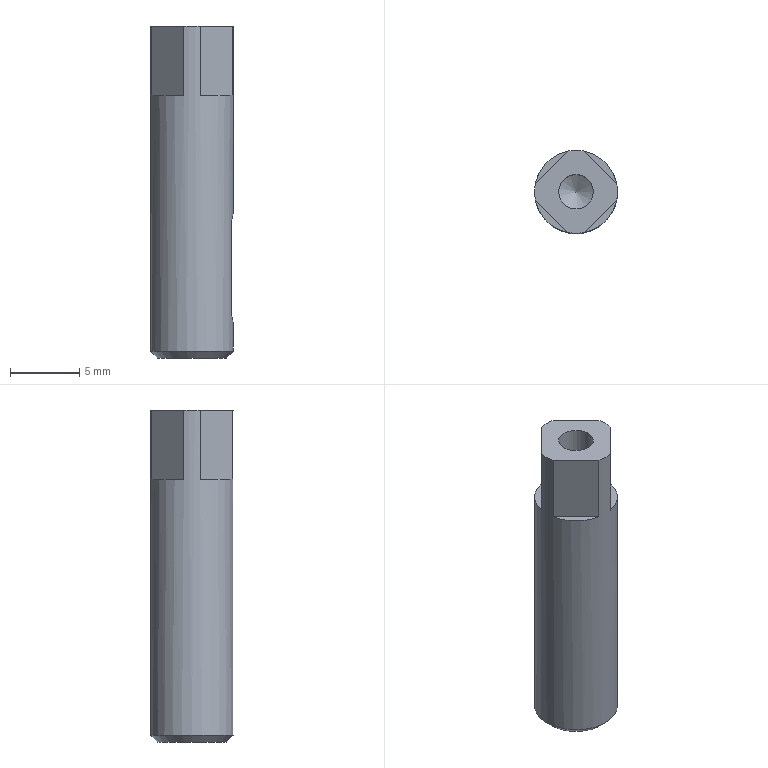Part | NX | features BREP 1 | 1 solid | 20 faces | box 6 x 6 x 24 mm | volume 581.313 mm3 | plane 13 | cylinder 5 | cone 2 | commonest cylinder face diameters 2 x2 2.5 x2 6 x1
STEP:
#1=CARTESIAN_POINT('',(-0.5952,-2.94,19.));
#2=VERTEX_POINT('',#1);
#3=CARTESIAN_POINT('',(-2.94,-0.5952,19.));
#4=VERTEX_POINT('',#3);
#5=CARTESIAN_POINT('',(-0.5952,-2.94,19.));
#6=DIRECTION('',(-0.7071,0.7071,0.));
#7=VECTOR('',#6,1000.);
#8=LINE('',#5,#7);
#9=EDGE_CURVE('',#2,#4,#8,.T.);
#10=ORIENTED_EDGE('',*,*,#9,.T.);
#11=CARTESIAN_POINT('',(0.,0.,19.));
#12=DIRECTION('',(0.,0.,1.));
#13=DIRECTION('',(-0.9801,-0.1984,0.));
#14=AXIS2_PLACEMENT_3D('',#11,#12,#13);
#15=CIRCLE('',#14,3.);
#16=EDGE_CURVE('',#4,#2,#15,.T.);
#17=ORIENTED_EDGE('',*,*,#16,.T.);
#18=EDGE_LOOP('',(#10,#17));
#19=FACE_BOUND('',#18,.T.);
#20=CARTESIAN_POINT('',(0.,0.,19.));
#21=DIRECTION('',(0.,0.,1.));
#22=DIRECTION('',(-1.,0.,0.));
#23=AXIS2_PLACEMENT_3D('',#20,#21,#22);
#24=PLANE('',#23);
#25=ADVANCED_FACE('',(#19),#24,.T.);
#26=CARTESIAN_POINT('',(2.94,-0.5952,19.));
#27=VERTEX_POINT('',#26);
#28=CARTESIAN_POINT('',(0.5952,-2.94,19.));
#29=VERTEX_POINT('',#28);
#30=CARTESIAN_POINT('',(2.94,-0.5952,19.));
#31=DIRECTION('',(-0.7071,-0.7071,0.));
#32=VECTOR('',#31,1000.);
#33=LINE('',#30,#32);
#34=EDGE_CURVE('',#27,#29,#33,.T.);
#35=ORIENTED_EDGE('',*,*,#34,.T.);
#36=CARTESIAN_POINT('',(0.,0.,19.));
#37=DIRECTION('',(0.,0.,1.));
#38=DIRECTION('',(0.1984,-0.9801,0.));
#39=AXIS2_PLACEMENT_3D('',#36,#37,#38);
#40=CIRCLE('',#39,3.);
#41=EDGE_CURVE('',#29,#27,#40,.T.);
#42=ORIENTED_EDGE('',*,*,#41,.T.);
#43=EDGE_LOOP('',(#35,#42));
#44=FACE_BOUND('',#43,.T.);
#45=CARTESIAN_POINT('',(0.,0.,19.));
#46=DIRECTION('',(0.,0.,1.));
#47=DIRECTION('',(-1.,0.,0.));
#48=AXIS2_PLACEMENT_3D('',#45,#46,#47);
#49=PLANE('',#48);
#50=ADVANCED_FACE('',(#44),#49,.T.);
#51=CARTESIAN_POINT('',(0.5952,2.94,19.));
#52=VERTEX_POINT('',#51);
#53=CARTESIAN_POINT('',(2.94,0.5952,19.));
#54=VERTEX_POINT('',#53);
#55=CARTESIAN_POINT('',(0.5952,2.94,19.));
#56=DIRECTION('',(0.7071,-0.7071,0.));
#57=VECTOR('',#56,1000.);
#58=LINE('',#55,#57);
#59=EDGE_CURVE('',#52,#54,#58,.T.);
#60=ORIENTED_EDGE('',*,*,#59,.T.);
#61=CARTESIAN_POINT('',(0.,0.,19.));
#62=DIRECTION('',(0.,0.,1.));
#63=DIRECTION('',(0.9801,0.1984,0.));
#64=AXIS2_PLACEMENT_3D('',#61,#62,#63);
#65=CIRCLE('',#64,3.);
#66=EDGE_CURVE('',#54,#52,#65,.T.);
#67=ORIENTED_EDGE('',*,*,#66,.T.);
#68=EDGE_LOOP('',(#60,#67));
#69=FACE_BOUND('',#68,.T.);
#70=CARTESIAN_POINT('',(0.,0.,19.));
#71=DIRECTION('',(0.,0.,1.));
#72=DIRECTION('',(-1.,0.,0.));
#73=AXIS2_PLACEMENT_3D('',#70,#71,#72);
#74=PLANE('',#73);
#75=ADVANCED_FACE('',(#69),#74,.T.);
#76=CARTESIAN_POINT('',(-2.94,0.5952,19.));
#77=VERTEX_POINT('',#76);
#78=CARTESIAN_POINT('',(-0.5952,2.94,19.));
#79=VERTEX_POINT('',#78);
#80=CARTESIAN_POINT('',(-2.94,0.5952,19.));
#81=DIRECTION('',(0.7071,0.7071,0.));
#82=VECTOR('',#81,1000.);
#83=LINE('',#80,#82);
#84=EDGE_CURVE('',#77,#79,#83,.T.);
#85=ORIENTED_EDGE('',*,*,#84,.T.);
#86=CARTESIAN_POINT('',(0.,0.,19.));
#87=DIRECTION('',(0.,0.,1.));
#88=DIRECTION('',(-0.1984,0.9801,0.));
#89=AXIS2_PLACEMENT_3D('',#86,#87,#88);
#90=CIRCLE('',#89,3.);
#91=EDGE_CURVE('',#79,#77,#90,.T.);
#92=ORIENTED_EDGE('',*,*,#91,.T.);
#93=EDGE_LOOP('',(#85,#92));
#94=FACE_BOUND('',#93,.T.);
#95=CARTESIAN_POINT('',(0.,0.,19.));
#96=DIRECTION('',(0.,0.,1.));
#97=DIRECTION('',(-1.,0.,0.));
#98=AXIS2_PLACEMENT_3D('',#95,#96,#97);
#99=PLANE('',#98);
#100=ADVANCED_FACE('',(#94),#99,.T.);
#101=CARTESIAN_POINT('',(-0.5952,-2.94,24.));
#102=VERTEX_POINT('',#101);
#103=CARTESIAN_POINT('',(-2.94,-0.5952,24.));
#104=VERTEX_POINT('',#103);
#105=CARTESIAN_POINT('',(-0.5952,-2.94,24.));
#106=DIRECTION('',(-0.7071,0.7071,0.));
#107=VECTOR('',#106,1000.);
#108=LINE('',#105,#107);
#109=EDGE_CURVE('',#102,#104,#108,.T.);
#110=ORIENTED_EDGE('',*,*,#109,.T.);
#111=CARTESIAN_POINT('',(-2.94,-0.5952,24.));
#112=DIRECTION('',(0.,0.,-1.));
#113=VECTOR('',#112,1000.);
#114=LINE('',#111,#113);
#115=EDGE_CURVE('',#104,#4,#114,.T.);
#116=ORIENTED_EDGE('',*,*,#115,.T.);
#117=ORIENTED_EDGE('',*,*,#9,.F.);
#118=CARTESIAN_POINT('',(-0.5952,-2.94,19.));
#119=DIRECTION('',(0.,0.,1.));
#120=VECTOR('',#119,1000.);
#121=LINE('',#118,#120);
#122=EDGE_CURVE('',#2,#102,#121,.T.);
#123=ORIENTED_EDGE('',*,*,#122,.T.);
#124=EDGE_LOOP('',(#110,#116,#117,#123));
#125=FACE_BOUND('',#124,.T.);
#126=CARTESIAN_POINT('',(-1.768,-1.768,21.5));
#127=DIRECTION('',(-0.7071,-0.7071,0.));
#128=DIRECTION('',(0.7071,-0.7071,0.));
#129=AXIS2_PLACEMENT_3D('',#126,#127,#128);
#130=PLANE('',#129);
#131=ADVANCED_FACE('',(#125),#130,.T.);
#132=CARTESIAN_POINT('',(-2.94,0.5952,24.));
#133=VERTEX_POINT('',#132);
#134=CARTESIAN_POINT('',(-0.5952,2.94,24.));
#135=VERTEX_POINT('',#134);
#136=CARTESIAN_POINT('',(-2.94,0.5952,24.));
#137=DIRECTION('',(0.7071,0.7071,0.));
#138=VECTOR('',#137,1000.);
#139=LINE('',#136,#138);
#140=EDGE_CURVE('',#133,#135,#139,.T.);
#141=ORIENTED_EDGE('',*,*,#140,.T.);
#142=CARTESIAN_POINT('',(-0.5952,2.94,24.));
#143=DIRECTION('',(0.,0.,-1.));
#144=VECTOR('',#143,1000.);
#145=LINE('',#142,#144);
#146=EDGE_CURVE('',#135,#79,#145,.T.);
#147=ORIENTED_EDGE('',*,*,#146,.T.);
#148=ORIENTED_EDGE('',*,*,#84,.F.);
#149=CARTESIAN_POINT('',(-2.94,0.5952,19.));
#150=DIRECTION('',(0.,0.,1.));
#151=VECTOR('',#150,1000.);
#152=LINE('',#149,#151);
#153=EDGE_CURVE('',#77,#133,#152,.T.);
#154=ORIENTED_EDGE('',*,*,#153,.T.);
#155=EDGE_LOOP('',(#141,#147,#148,#154));
#156=FACE_BOUND('',#155,.T.);
#157=CARTESIAN_POINT('',(-1.768,1.768,21.5));
#158=DIRECTION('',(-0.7071,0.7071,0.));
#159=DIRECTION('',(-0.7071,-0.7071,0.));
#160=AXIS2_PLACEMENT_3D('',#157,#158,#159);
#161=PLANE('',#160);
#162=ADVANCED_FACE('',(#156),#161,.T.);
#163=CARTESIAN_POINT('',(0.5952,2.94,24.));
#164=VERTEX_POINT('',#163);
#165=CARTESIAN_POINT('',(2.94,0.5952,24.));
#166=VERTEX_POINT('',#165);
#167=CARTESIAN_POINT('',(0.5952,2.94,24.));
#168=DIRECTION('',(0.7071,-0.7071,0.));
#169=VECTOR('',#168,1000.);
#170=LINE('',#167,#169);
#171=EDGE_CURVE('',#164,#166,#170,.T.);
#172=ORIENTED_EDGE('',*,*,#171,.T.);
#173=CARTESIAN_POINT('',(2.94,0.5952,24.));
#174=DIRECTION('',(0.,0.,-1.));
#175=VECTOR('',#174,1000.);
#176=LINE('',#173,#175);
#177=EDGE_CURVE('',#166,#54,#176,.T.);
#178=ORIENTED_EDGE('',*,*,#177,.T.);
#179=ORIENTED_EDGE('',*,*,#59,.F.);
#180=CARTESIAN_POINT('',(0.5952,2.94,19.));
#181=DIRECTION('',(0.,0.,1.));
#182=VECTOR('',#181,1000.);
#183=LINE('',#180,#182);
#184=EDGE_CURVE('',#52,#164,#183,.T.);
#185=ORIENTED_EDGE('',*,*,#184,.T.);
#186=EDGE_LOOP('',(#172,#178,#179,#185));
#187=FACE_BOUND('',#186,.T.);
#188=CARTESIAN_POINT('',(1.768,1.768,21.5));
#189=DIRECTION('',(0.7071,0.7071,0.));
#190=DIRECTION('',(-0.7071,0.7071,0.));
#191=AXIS2_PLACEMENT_3D('',#188,#189,#190);
#192=PLANE('',#191);
#193=ADVANCED_FACE('',(#187),#192,.T.);
#194=CARTESIAN_POINT('',(2.94,-0.5952,24.));
#195=VERTEX_POINT('',#194);
#196=CARTESIAN_POINT('',(0.5952,-2.94,24.));
#197=VERTEX_POINT('',#196);
#198=CARTESIAN_POINT('',(2.94,-0.5952,24.));
#199=DIRECTION('',(-0.7071,-0.7071,0.));
#200=VECTOR('',#199,1000.);
#201=LINE('',#198,#200);
#202=EDGE_CURVE('',#195,#197,#201,.T.);
#203=ORIENTED_EDGE('',*,*,#202,.T.);
#204=CARTESIAN_POINT('',(0.5952,-2.94,24.));
#205=DIRECTION('',(0.,0.,-1.));
#206=VECTOR('',#205,1000.);
#207=LINE('',#204,#206);
#208=EDGE_CURVE('',#197,#29,#207,.T.);
#209=ORIENTED_EDGE('',*,*,#208,.T.);
#210=ORIENTED_EDGE('',*,*,#34,.F.);
#211=CARTESIAN_POINT('',(2.94,-0.5952,19.));
#212=DIRECTION('',(0.,0.,1.));
#213=VECTOR('',#212,1000.);
#214=LINE('',#211,#213);
#215=EDGE_CURVE('',#27,#195,#214,.T.);
#216=ORIENTED_EDGE('',*,*,#215,.T.);
#217=EDGE_LOOP('',(#203,#209,#210,#216));
#218=FACE_BOUND('',#217,.T.);
#219=CARTESIAN_POINT('',(1.768,-1.768,21.5));
#220=DIRECTION('',(0.7071,-0.7071,0.));
#221=DIRECTION('',(0.7071,0.7071,0.));
#222=AXIS2_PLACEMENT_3D('',#219,#220,#221);
#223=PLANE('',#222);
#224=ADVANCED_FACE('',(#218),#223,.T.);
#225=CARTESIAN_POINT('',(3.,0.,24.));
#226=VERTEX_POINT('',#225);
#227=CARTESIAN_POINT('',(0.,0.,24.));
#228=DIRECTION('',(0.,0.,1.));
#229=DIRECTION('',(0.9801,-0.1984,0.));
#230=AXIS2_PLACEMENT_3D('',#227,#228,#229);
#231=CIRCLE('',#230,3.);
#232=EDGE_CURVE('',#195,#226,#231,.T.);
#233=ORIENTED_EDGE('',*,*,#232,.F.);
#234=ORIENTED_EDGE('',*,*,#215,.F.);
#235=ORIENTED_EDGE('',*,*,#41,.F.);
#236=ORIENTED_EDGE('',*,*,#208,.F.);
#237=CARTESIAN_POINT('',(0.,0.,24.));
#238=DIRECTION('',(0.,0.,1.));
#239=DIRECTION('',(-0.1984,-0.9801,0.));
#240=AXIS2_PLACEMENT_3D('',#237,#238,#239);
#241=CIRCLE('',#240,3.);
#242=EDGE_CURVE('',#102,#197,#241,.T.);
#243=ORIENTED_EDGE('',*,*,#242,.F.);
#244=ORIENTED_EDGE('',*,*,#122,.F.);
#245=ORIENTED_EDGE('',*,*,#16,.F.);
#246=ORIENTED_EDGE('',*,*,#115,.F.);
#247=CARTESIAN_POINT('',(0.,0.,24.));
#248=DIRECTION('',(0.,0.,1.));
#249=DIRECTION('',(-0.9801,0.1984,0.));
#250=AXIS2_PLACEMENT_3D('',#247,#248,#249);
#251=CIRCLE('',#250,3.);
#252=EDGE_CURVE('',#133,#104,#251,.T.);
#253=ORIENTED_EDGE('',*,*,#252,.F.);
#254=ORIENTED_EDGE('',*,*,#153,.F.);
#255=ORIENTED_EDGE('',*,*,#91,.F.);
#256=ORIENTED_EDGE('',*,*,#146,.F.);
#257=CARTESIAN_POINT('',(0.,0.,24.));
#258=DIRECTION('',(0.,0.,1.));
#259=DIRECTION('',(0.1984,0.9801,0.));
#260=AXIS2_PLACEMENT_3D('',#257,#258,#259);
#261=CIRCLE('',#260,3.);
#262=EDGE_CURVE('',#164,#135,#261,.T.);
#263=ORIENTED_EDGE('',*,*,#262,.F.);
#264=ORIENTED_EDGE('',*,*,#184,.F.);
#265=ORIENTED_EDGE('',*,*,#66,.F.);
#266=ORIENTED_EDGE('',*,*,#177,.F.);
#267=CARTESIAN_POINT('',(0.,0.,24.));
#268=DIRECTION('',(0.,0.,1.));
#269=DIRECTION('',(1.,0.,0.));
#270=AXIS2_PLACEMENT_3D('',#267,#268,#269);
#271=CIRCLE('',#270,3.);
#272=EDGE_CURVE('',#226,#166,#271,.T.);
#273=ORIENTED_EDGE('',*,*,#272,.F.);
#274=CARTESIAN_POINT('',(3.,0.,10.5));
#275=VERTEX_POINT('',#274);
#276=CARTESIAN_POINT('',(3.,0.,10.5));
#277=DIRECTION('',(0.,0.,1.));
#278=VECTOR('',#277,1000.);
#279=LINE('',#276,#278);
#280=EDGE_CURVE('',#275,#226,#279,.T.);
#281=ORIENTED_EDGE('',*,*,#280,.F.);
#282=CARTESIAN_POINT('',(2.828,1.,9.5));
#283=VERTEX_POINT('',#282);
#284=CARTESIAN_POINT('',(2.828,1.,9.5));
#285=CARTESIAN_POINT('',(2.828,1.,10.032));
#286=CARTESIAN_POINT('',(3.,0.5323,10.5));
#287=CARTESIAN_POINT('',(3.,0.,10.5));
#288=B_SPLINE_CURVE_WITH_KNOTS('',3,(#284,#285,#286,#287),.UNSPECIFIED.,.F.,.F.,(4,4),(0.,0.001574),.UNSPECIFIED.);
#289=EDGE_CURVE('',#283,#275,#288,.T.);
#290=ORIENTED_EDGE('',*,*,#289,.F.);
#291=CARTESIAN_POINT('',(2.828,1.,3.5));
#292=VERTEX_POINT('',#291);
#293=CARTESIAN_POINT('',(2.828,1.,3.5));
#294=DIRECTION('',(0.,0.,1.));
#295=VECTOR('',#294,1000.);
#296=LINE('',#293,#295);
#297=EDGE_CURVE('',#292,#283,#296,.T.);
#298=ORIENTED_EDGE('',*,*,#297,.F.);
#299=CARTESIAN_POINT('',(3.,0.,2.5));
#300=VERTEX_POINT('',#299);
#301=CARTESIAN_POINT('',(3.,0.,2.5));
#302=CARTESIAN_POINT('',(3.,0.5323,2.5));
#303=CARTESIAN_POINT('',(2.828,1.,2.968));
#304=CARTESIAN_POINT('',(2.828,1.,3.5));
#305=B_SPLINE_CURVE_WITH_KNOTS('',3,(#301,#302,#303,#304),.UNSPECIFIED.,.F.,.F.,(4,4),(0.,0.001574),.UNSPECIFIED.);
#306=EDGE_CURVE('',#300,#292,#305,.T.);
#307=ORIENTED_EDGE('',*,*,#306,.F.);
#308=CARTESIAN_POINT('',(3.,0.,0.5));
#309=VERTEX_POINT('',#308);
#310=CARTESIAN_POINT('',(3.,0.,0.5));
#311=DIRECTION('',(0.,0.,1.));
#312=VECTOR('',#311,1000.);
#313=LINE('',#310,#312);
#314=EDGE_CURVE('',#309,#300,#313,.T.);
#315=ORIENTED_EDGE('',*,*,#314,.F.);
#316=CARTESIAN_POINT('',(0.,0.,0.5));
#317=DIRECTION('',(0.,0.,-1.));
#318=DIRECTION('',(1.,0.,0.));
#319=AXIS2_PLACEMENT_3D('',#316,#317,#318);
#320=CIRCLE('',#319,3.);
#321=EDGE_CURVE('',#309,#309,#320,.T.);
#322=ORIENTED_EDGE('',*,*,#321,.F.);
#323=ORIENTED_EDGE('',*,*,#314,.T.);
#324=CARTESIAN_POINT('',(2.828,-1.,3.5));
#325=VERTEX_POINT('',#324);
#326=CARTESIAN_POINT('',(2.828,-1.,3.5));
#327=CARTESIAN_POINT('',(2.828,-1.,2.968));
#328=CARTESIAN_POINT('',(3.,-0.5323,2.5));
#329=CARTESIAN_POINT('',(3.,0.,2.5));
#330=B_SPLINE_CURVE_WITH_KNOTS('',3,(#326,#327,#328,#329),.UNSPECIFIED.,.F.,.F.,(4,4),(0.,0.001574),.UNSPECIFIED.);
#331=EDGE_CURVE('',#325,#300,#330,.T.);
#332=ORIENTED_EDGE('',*,*,#331,.F.);
#333=CARTESIAN_POINT('',(2.828,-1.,9.5));
#334=VERTEX_POINT('',#333);
#335=CARTESIAN_POINT('',(2.828,-1.,9.5));
#336=DIRECTION('',(0.,0.,-1.));
#337=VECTOR('',#336,1000.);
#338=LINE('',#335,#337);
#339=EDGE_CURVE('',#334,#325,#338,.T.);
#340=ORIENTED_EDGE('',*,*,#339,.F.);
#341=CARTESIAN_POINT('',(3.,0.,10.5));
#342=CARTESIAN_POINT('',(3.,-0.5323,10.5));
#343=CARTESIAN_POINT('',(2.828,-1.,10.032));
#344=CARTESIAN_POINT('',(2.828,-1.,9.5));
#345=B_SPLINE_CURVE_WITH_KNOTS('',3,(#341,#342,#343,#344),.UNSPECIFIED.,.F.,.F.,(4,4),(0.,0.001574),.UNSPECIFIED.);
#346=EDGE_CURVE('',#275,#334,#345,.T.);
#347=ORIENTED_EDGE('',*,*,#346,.F.);
#348=ORIENTED_EDGE('',*,*,#280,.T.);
#349=EDGE_LOOP('',(#233,#234,#235,#236,#243,#244,#245,#246,#253,#254,#255,#256,#263,#264,#265,#266,#273,#281,#290,#298,#307,#315,#322,#323,#332,#340,#347,#348));
#350=FACE_BOUND('',#349,.T.);
#351=CARTESIAN_POINT('',(0.,0.,0.));
#352=DIRECTION('',(0.,0.,1.));
#353=DIRECTION('',(-1.,0.,0.));
#354=AXIS2_PLACEMENT_3D('',#351,#352,#353);
#355=CYLINDRICAL_SURFACE('',#354,3.);
#356=ADVANCED_FACE('',(#350),#355,.T.);
#357=ORIENTED_EDGE('',*,*,#272,.T.);
#358=ORIENTED_EDGE('',*,*,#171,.F.);
#359=ORIENTED_EDGE('',*,*,#262,.T.);
#360=ORIENTED_EDGE('',*,*,#140,.F.);
#361=ORIENTED_EDGE('',*,*,#252,.T.);
#362=ORIENTED_EDGE('',*,*,#109,.F.);
#363=ORIENTED_EDGE('',*,*,#242,.T.);
#364=ORIENTED_EDGE('',*,*,#202,.F.);
#365=ORIENTED_EDGE('',*,*,#232,.T.);
#366=EDGE_LOOP('',(#357,#358,#359,#360,#361,#362,#363,#364,#365));
#367=FACE_BOUND('',#366,.T.);
#368=CARTESIAN_POINT('',(1.25,0.,24.));
#369=VERTEX_POINT('',#368);
#370=CARTESIAN_POINT('',(0.,0.,24.));
#371=DIRECTION('',(0.,0.,-1.));
#372=DIRECTION('',(1.,0.,0.));
#373=AXIS2_PLACEMENT_3D('',#370,#371,#372);
#374=CIRCLE('',#373,1.25);
#375=EDGE_CURVE('',#369,#369,#374,.T.);
#376=ORIENTED_EDGE('',*,*,#375,.T.);
#377=EDGE_LOOP('',(#376));
#378=FACE_BOUND('',#377,.T.);
#379=CARTESIAN_POINT('',(0.,0.,24.));
#380=DIRECTION('',(0.,0.,1.));
#381=DIRECTION('',(-1.,0.,0.));
#382=AXIS2_PLACEMENT_3D('',#379,#380,#381);
#383=PLANE('',#382);
#384=ADVANCED_FACE('',(#367,#378),#383,.T.);
#385=CARTESIAN_POINT('',(2.5,0.,0.));
#386=VERTEX_POINT('',#385);
#387=CARTESIAN_POINT('',(0.,0.,0.));
#388=DIRECTION('',(0.,0.,-1.));
#389=DIRECTION('',(1.,0.,0.));
#390=AXIS2_PLACEMENT_3D('',#387,#388,#389);
#391=CIRCLE('',#390,2.5);
#392=EDGE_CURVE('',#386,#386,#391,.T.);
#393=ORIENTED_EDGE('',*,*,#392,.T.);
#394=EDGE_LOOP('',(#393));
#395=FACE_BOUND('',#394,.T.);
#396=CARTESIAN_POINT('',(0.,0.,0.));
#397=DIRECTION('',(0.,0.,1.));
#398=DIRECTION('',(-1.,0.,0.));
#399=AXIS2_PLACEMENT_3D('',#396,#397,#398);
#400=PLANE('',#399);
#401=ADVANCED_FACE('',(#395),#400,.F.);
#402=ORIENTED_EDGE('',*,*,#392,.F.);
#403=CARTESIAN_POINT('',(2.5,0.,0.));
#404=DIRECTION('',(0.7071,0.,0.7071));
#405=VECTOR('',#404,1000.);
#406=LINE('',#403,#405);
#407=EDGE_CURVE('',#386,#309,#406,.T.);
#408=ORIENTED_EDGE('',*,*,#407,.T.);
#409=ORIENTED_EDGE('',*,*,#321,.T.);
#410=ORIENTED_EDGE('',*,*,#407,.F.);
#411=EDGE_LOOP('',(#402,#408,#409,#410));
#412=FACE_BOUND('',#411,.T.);
#413=CARTESIAN_POINT('',(0.,0.,0.));
#414=DIRECTION('',(0.,0.,1.));
#415=DIRECTION('',(-1.,0.,0.));
#416=AXIS2_PLACEMENT_3D('',#413,#414,#415);
#417=CONICAL_SURFACE('',#416,2.5,0.7854);
#418=ADVANCED_FACE('',(#412),#417,.T.);
#419=CARTESIAN_POINT('',(1.8,1.,9.5));
#420=VERTEX_POINT('',#419);
#421=CARTESIAN_POINT('',(1.8,1.,9.5));
#422=DIRECTION('',(1.,0.,0.));
#423=VECTOR('',#422,1000.);
#424=LINE('',#421,#423);
#425=EDGE_CURVE('',#420,#283,#424,.T.);
#426=ORIENTED_EDGE('',*,*,#425,.T.);
#427=ORIENTED_EDGE('',*,*,#289,.T.);
#428=ORIENTED_EDGE('',*,*,#346,.T.);
#429=CARTESIAN_POINT('',(1.8,-1.,9.5));
#430=VERTEX_POINT('',#429);
#431=CARTESIAN_POINT('',(1.8,-1.,9.5));
#432=DIRECTION('',(1.,0.,0.));
#433=VECTOR('',#432,1000.);
#434=LINE('',#431,#433);
#435=EDGE_CURVE('',#430,#334,#434,.T.);
#436=ORIENTED_EDGE('',*,*,#435,.F.);
#437=CARTESIAN_POINT('',(1.8,0.,9.5));
#438=DIRECTION('',(1.,0.,0.));
#439=DIRECTION('',(0.,1.,0.));
#440=AXIS2_PLACEMENT_3D('',#437,#438,#439);
#441=CIRCLE('',#440,1.);
#442=EDGE_CURVE('',#420,#430,#441,.T.);
#443=ORIENTED_EDGE('',*,*,#442,.F.);
#444=EDGE_LOOP('',(#426,#427,#428,#436,#443));
#445=FACE_BOUND('',#444,.T.);
#446=CARTESIAN_POINT('',(1.8,0.,9.5));
#447=DIRECTION('',(1.,0.,0.));
#448=DIRECTION('',(0.,-1.,0.));
#449=AXIS2_PLACEMENT_3D('',#446,#447,#448);
#450=CYLINDRICAL_SURFACE('',#449,1.);
#451=ADVANCED_FACE('',(#445),#450,.F.);
#452=CARTESIAN_POINT('',(1.8,1.,3.5));
#453=VERTEX_POINT('',#452);
#454=CARTESIAN_POINT('',(1.8,1.,3.5));
#455=DIRECTION('',(1.,0.,0.));
#456=VECTOR('',#455,1000.);
#457=LINE('',#454,#456);
#458=EDGE_CURVE('',#453,#292,#457,.T.);
#459=ORIENTED_EDGE('',*,*,#458,.T.);
#460=ORIENTED_EDGE('',*,*,#297,.T.);
#461=ORIENTED_EDGE('',*,*,#425,.F.);
#462=CARTESIAN_POINT('',(1.8,1.,3.5));
#463=DIRECTION('',(0.,0.,1.));
#464=VECTOR('',#463,1000.);
#465=LINE('',#462,#464);
#466=EDGE_CURVE('',#453,#420,#465,.T.);
#467=ORIENTED_EDGE('',*,*,#466,.F.);
#468=EDGE_LOOP('',(#459,#460,#461,#467));
#469=FACE_BOUND('',#468,.T.);
#470=CARTESIAN_POINT('',(4.805,1.,6.5));
#471=DIRECTION('',(0.,1.,0.));
#472=DIRECTION('',(0.,0.,-1.));
#473=AXIS2_PLACEMENT_3D('',#470,#471,#472);
#474=PLANE('',#473);
#475=ADVANCED_FACE('',(#469),#474,.F.);
#476=CARTESIAN_POINT('',(1.8,-1.,3.5));
#477=VERTEX_POINT('',#476);
#478=CARTESIAN_POINT('',(1.8,-1.,3.5));
#479=DIRECTION('',(1.,0.,0.));
#480=VECTOR('',#479,1000.);
#481=LINE('',#478,#480);
#482=EDGE_CURVE('',#477,#325,#481,.T.);
#483=ORIENTED_EDGE('',*,*,#482,.T.);
#484=ORIENTED_EDGE('',*,*,#331,.T.);
#485=ORIENTED_EDGE('',*,*,#306,.T.);
#486=ORIENTED_EDGE('',*,*,#458,.F.);
#487=CARTESIAN_POINT('',(1.8,0.,3.5));
#488=DIRECTION('',(1.,0.,0.));
#489=DIRECTION('',(0.,-1.,0.));
#490=AXIS2_PLACEMENT_3D('',#487,#488,#489);
#491=CIRCLE('',#490,1.);
#492=EDGE_CURVE('',#477,#453,#491,.T.);
#493=ORIENTED_EDGE('',*,*,#492,.F.);
#494=EDGE_LOOP('',(#483,#484,#485,#486,#493));
#495=FACE_BOUND('',#494,.T.);
#496=CARTESIAN_POINT('',(1.8,0.,3.5));
#497=DIRECTION('',(1.,0.,0.));
#498=DIRECTION('',(0.,1.,0.));
#499=AXIS2_PLACEMENT_3D('',#496,#497,#498);
#500=CYLINDRICAL_SURFACE('',#499,1.);
#501=ADVANCED_FACE('',(#495),#500,.F.);
#502=ORIENTED_EDGE('',*,*,#435,.T.);
#503=ORIENTED_EDGE('',*,*,#339,.T.);
#504=ORIENTED_EDGE('',*,*,#482,.F.);
#505=CARTESIAN_POINT('',(1.8,-1.,9.5));
#506=DIRECTION('',(0.,0.,-1.));
#507=VECTOR('',#506,1000.);
#508=LINE('',#505,#507);
#509=EDGE_CURVE('',#430,#477,#508,.T.);
#510=ORIENTED_EDGE('',*,*,#509,.F.);
#511=EDGE_LOOP('',(#502,#503,#504,#510));
#512=FACE_BOUND('',#511,.T.);
#513=CARTESIAN_POINT('',(4.805,-1.,6.5));
#514=DIRECTION('',(0.,-1.,0.));
#515=DIRECTION('',(0.,0.,1.));
#516=AXIS2_PLACEMENT_3D('',#513,#514,#515);
#517=PLANE('',#516);
#518=ADVANCED_FACE('',(#512),#517,.F.);
#519=ORIENTED_EDGE('',*,*,#442,.T.);
#520=ORIENTED_EDGE('',*,*,#509,.T.);
#521=ORIENTED_EDGE('',*,*,#492,.T.);
#522=ORIENTED_EDGE('',*,*,#466,.T.);
#523=EDGE_LOOP('',(#519,#520,#521,#522));
#524=FACE_BOUND('',#523,.T.);
#525=CARTESIAN_POINT('',(1.8,3.,6.5));
#526=DIRECTION('',(1.,0.,0.));
#527=DIRECTION('',(0.,-1.,0.));
#528=AXIS2_PLACEMENT_3D('',#525,#526,#527);
#529=PLANE('',#528);
#530=ADVANCED_FACE('',(#524),#529,.T.);
#531=CARTESIAN_POINT('',(1.25,0.,15.));
#532=VERTEX_POINT('',#531);
#533=CARTESIAN_POINT('',(1.25,0.,24.));
#534=DIRECTION('',(0.,0.,-1.));
#535=VECTOR('',#534,1000.);
#536=LINE('',#533,#535);
#537=EDGE_CURVE('',#369,#532,#536,.T.);
#538=ORIENTED_EDGE('',*,*,#537,.T.);
#539=CARTESIAN_POINT('',(0.,0.,15.));
#540=DIRECTION('',(0.,0.,-1.));
#541=DIRECTION('',(1.,0.,0.));
#542=AXIS2_PLACEMENT_3D('',#539,#540,#541);
#543=CIRCLE('',#542,1.25);
#544=EDGE_CURVE('',#532,#532,#543,.T.);
#545=ORIENTED_EDGE('',*,*,#544,.T.);
#546=ORIENTED_EDGE('',*,*,#537,.F.);
#547=ORIENTED_EDGE('',*,*,#375,.F.);
#548=EDGE_LOOP('',(#538,#545,#546,#547));
#549=FACE_BOUND('',#548,.T.);
#550=CARTESIAN_POINT('',(0.,0.,24.));
#551=DIRECTION('',(0.,0.,-1.));
#552=DIRECTION('',(-1.,0.,0.));
#553=AXIS2_PLACEMENT_3D('',#550,#551,#552);
#554=CYLINDRICAL_SURFACE('',#553,1.25);
#555=ADVANCED_FACE('',(#549),#554,.F.);
#556=CARTESIAN_POINT('',(1.25,0.,13.));
#557=VERTEX_POINT('',#556);
#558=CARTESIAN_POINT('',(1.25,0.,15.));
#559=DIRECTION('',(0.,0.,-1.));
#560=VECTOR('',#559,1000.);
#561=LINE('',#558,#560);
#562=EDGE_CURVE('',#532,#557,#561,.T.);
#563=ORIENTED_EDGE('',*,*,#562,.T.);
#564=CARTESIAN_POINT('',(0.,0.,13.));
#565=DIRECTION('',(0.,0.,-1.));
#566=DIRECTION('',(1.,0.,0.));
#567=AXIS2_PLACEMENT_3D('',#564,#565,#566);
#568=CIRCLE('',#567,1.25);
#569=EDGE_CURVE('',#557,#557,#568,.T.);
#570=ORIENTED_EDGE('',*,*,#569,.T.);
#571=ORIENTED_EDGE('',*,*,#562,.F.);
#572=ORIENTED_EDGE('',*,*,#544,.F.);
#573=EDGE_LOOP('',(#563,#570,#571,#572));
#574=FACE_BOUND('',#573,.T.);
#575=CARTESIAN_POINT('',(0.,0.,15.));
#576=DIRECTION('',(0.,0.,-1.));
#577=DIRECTION('',(-1.,0.,0.));
#578=AXIS2_PLACEMENT_3D('',#575,#576,#577);
#579=CYLINDRICAL_SURFACE('',#578,1.25);
#580=ADVANCED_FACE('',(#574),#579,.F.);
#581=CARTESIAN_POINT('',(0.,0.,12.249));
#582=VERTEX_POINT('',#581);
#583=CARTESIAN_POINT('',(1.25,0.,13.));
#584=DIRECTION('',(-0.8572,0.,-0.515));
#585=VECTOR('',#584,1000.);
#586=LINE('',#583,#585);
#587=EDGE_CURVE('',#557,#582,#586,.T.);
#588=ORIENTED_EDGE('',*,*,#587,.T.);
#589=ORIENTED_EDGE('',*,*,#587,.F.);
#590=ORIENTED_EDGE('',*,*,#569,.F.);
#591=EDGE_LOOP('',(#588,#589,#590));
#592=FACE_BOUND('',#591,.T.);
#593=CARTESIAN_POINT('',(0.,0.,12.249));
#594=DIRECTION('',(0.,0.,1.));
#595=DIRECTION('',(-1.,0.,0.));
#596=AXIS2_PLACEMENT_3D('',#593,#594,#595);
#597=CONICAL_SURFACE('',#596,0.,1.03);
#598=ADVANCED_FACE('',(#592),#597,.F.);
#599=CLOSED_SHELL('',(#25,#50,#75,#100,#131,#162,#193,#224,#356,#384,#401,#418,#451,#475,#501,#518,#530,#555,#580,#598));
#600=MANIFOLD_SOLID_BREP('',#599);
#601=(LENGTH_UNIT()NAMED_UNIT(*)SI_UNIT(.MILLI.,.METRE.));
#602=UNCERTAINTY_MEASURE_WITH_UNIT(LENGTH_MEASURE(0.0508),#601,'','');
#603=(NAMED_UNIT(*)PLANE_ANGLE_UNIT()SI_UNIT($,.RADIAN.));
#604=(NAMED_UNIT(*)SI_UNIT($,.STERADIAN.)SOLID_ANGLE_UNIT());
#605=(GEOMETRIC_REPRESENTATION_CONTEXT(3)GLOBAL_UNCERTAINTY_ASSIGNED_CONTEXT((#602))GLOBAL_UNIT_ASSIGNED_CONTEXT((#601,#603,#604))REPRESENTATION_CONTEXT('',''));
#606=ADVANCED_BREP_SHAPE_REPRESENTATION('',(#600),#605);